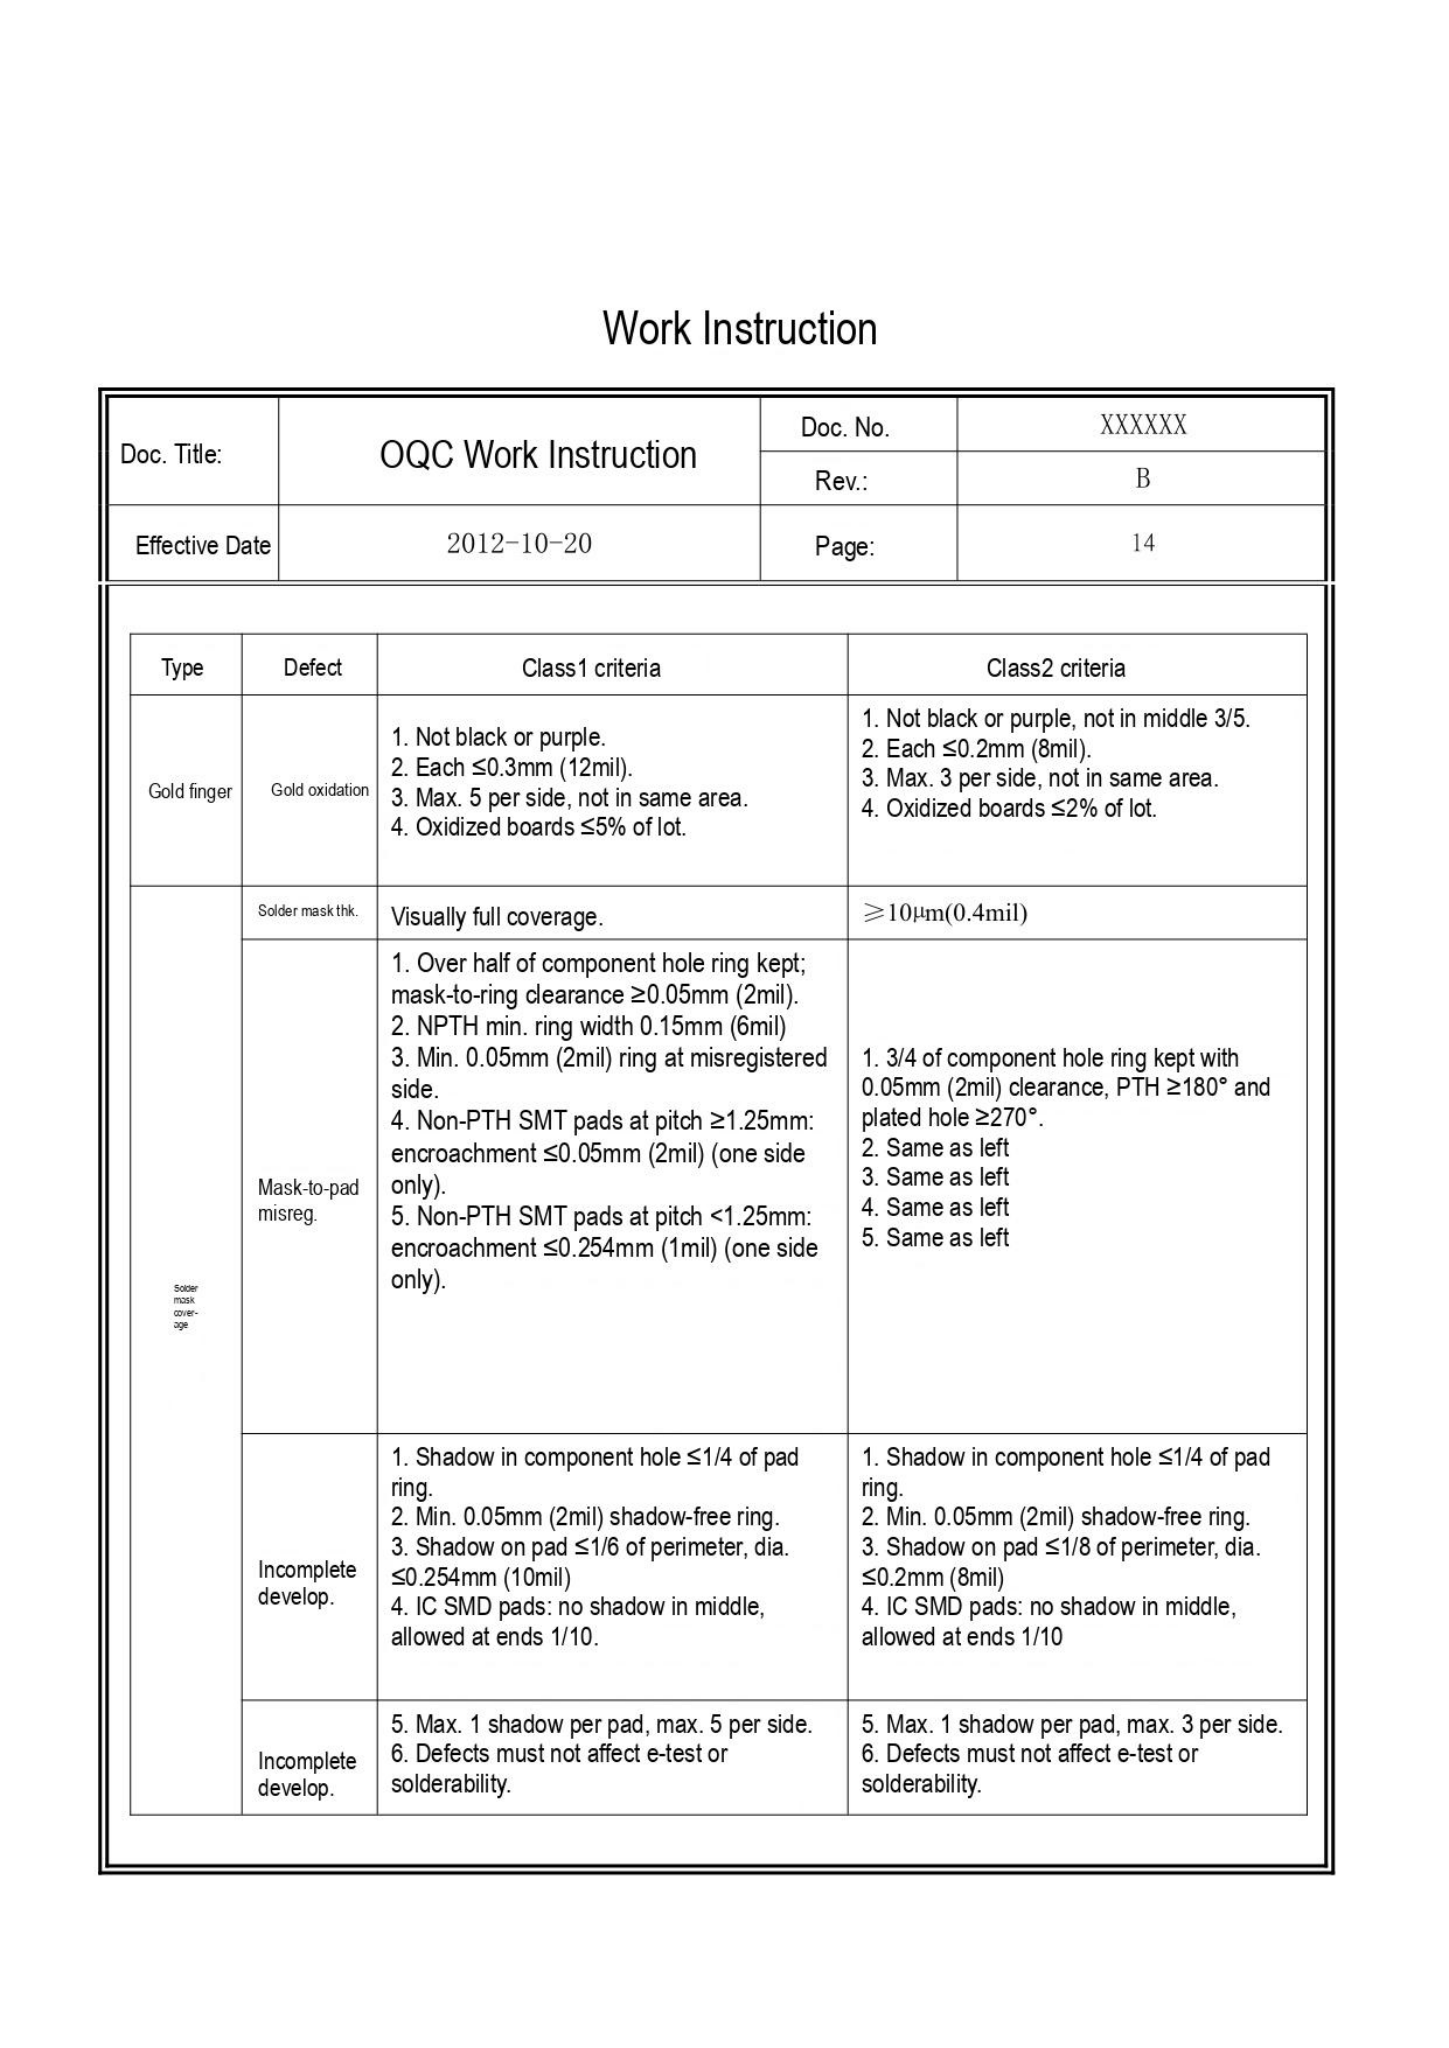Work Instruction

| Doc. Title: | OQC Work Instruction | Doc. No. | XXXXXX |
|---|---|---|---|
| | | Rev.: | B |
| Effective Date | 2012-10-20 | Page: | 14 |

| Type | Defect | Class1 criteria | Class2 criteria |
|---|---|---|---|
| Gold finger | Gold oxidation | 1. Not black or purple.<br>2. Each ≤0.3mm (12mil).<br>3. Max. 5 per side, not in same area.<br>4. Oxidized boards ≤5% of lot. | 1. Not black or purple, not in middle 3/5.<br>2. Each ≤0.2mm (8mil).<br>3. Max. 3 per side, not in same area.<br>4. Oxidized boards ≤2% of lot. |
| Solder mask cover-age | Solder mask thk. | Visually full coverage. | ≥10μm(0.4mil) |
| | Mask-to-pad misreg. | 1. Over half of component hole ring kept; mask-to-ring clearance ≥0.05mm (2mil).<br>2. NPTH min. ring width 0.15mm (6mil)<br>3. Min. 0.05mm (2mil) ring at misregistered side.<br>4. Non-PTH SMT pads at pitch ≥1.25mm: encroachment ≤0.05mm (2mil) (one side only).<br>5. Non-PTH SMT pads at pitch <1.25mm: encroachment ≤0.254mm (1mil) (one side only). | 1. 3/4 of component hole ring kept with 0.05mm (2mil) clearance, PTH ≥180° and plated hole ≥270°.<br>2. Same as left<br>3. Same as left<br>4. Same as left<br>5. Same as left |
| | Incomplete develop. | 1. Shadow in component hole ≤1/4 of pad ring.<br>2. Min. 0.05mm (2mil) shadow-free ring.<br>3. Shadow on pad ≤1/6 of perimeter, dia. ≤0.254mm (10mil)<br>4. IC SMD pads: no shadow in middle, allowed at ends 1/10. | 1. Shadow in component hole ≤1/4 of pad ring.<br>2. Min. 0.05mm (2mil) shadow-free ring.<br>3. Shadow on pad ≤1/8 of perimeter, dia. ≤0.2mm (8mil)<br>4. IC SMD pads: no shadow in middle, allowed at ends 1/10 |
| | Incomplete develop. | 5. Max. 1 shadow per pad, max. 5 per side.<br>6. Defects must not affect e-test or solderability. | 5. Max. 1 shadow per pad, max. 3 per side.<br>6. Defects must not affect e-test or solderability. |
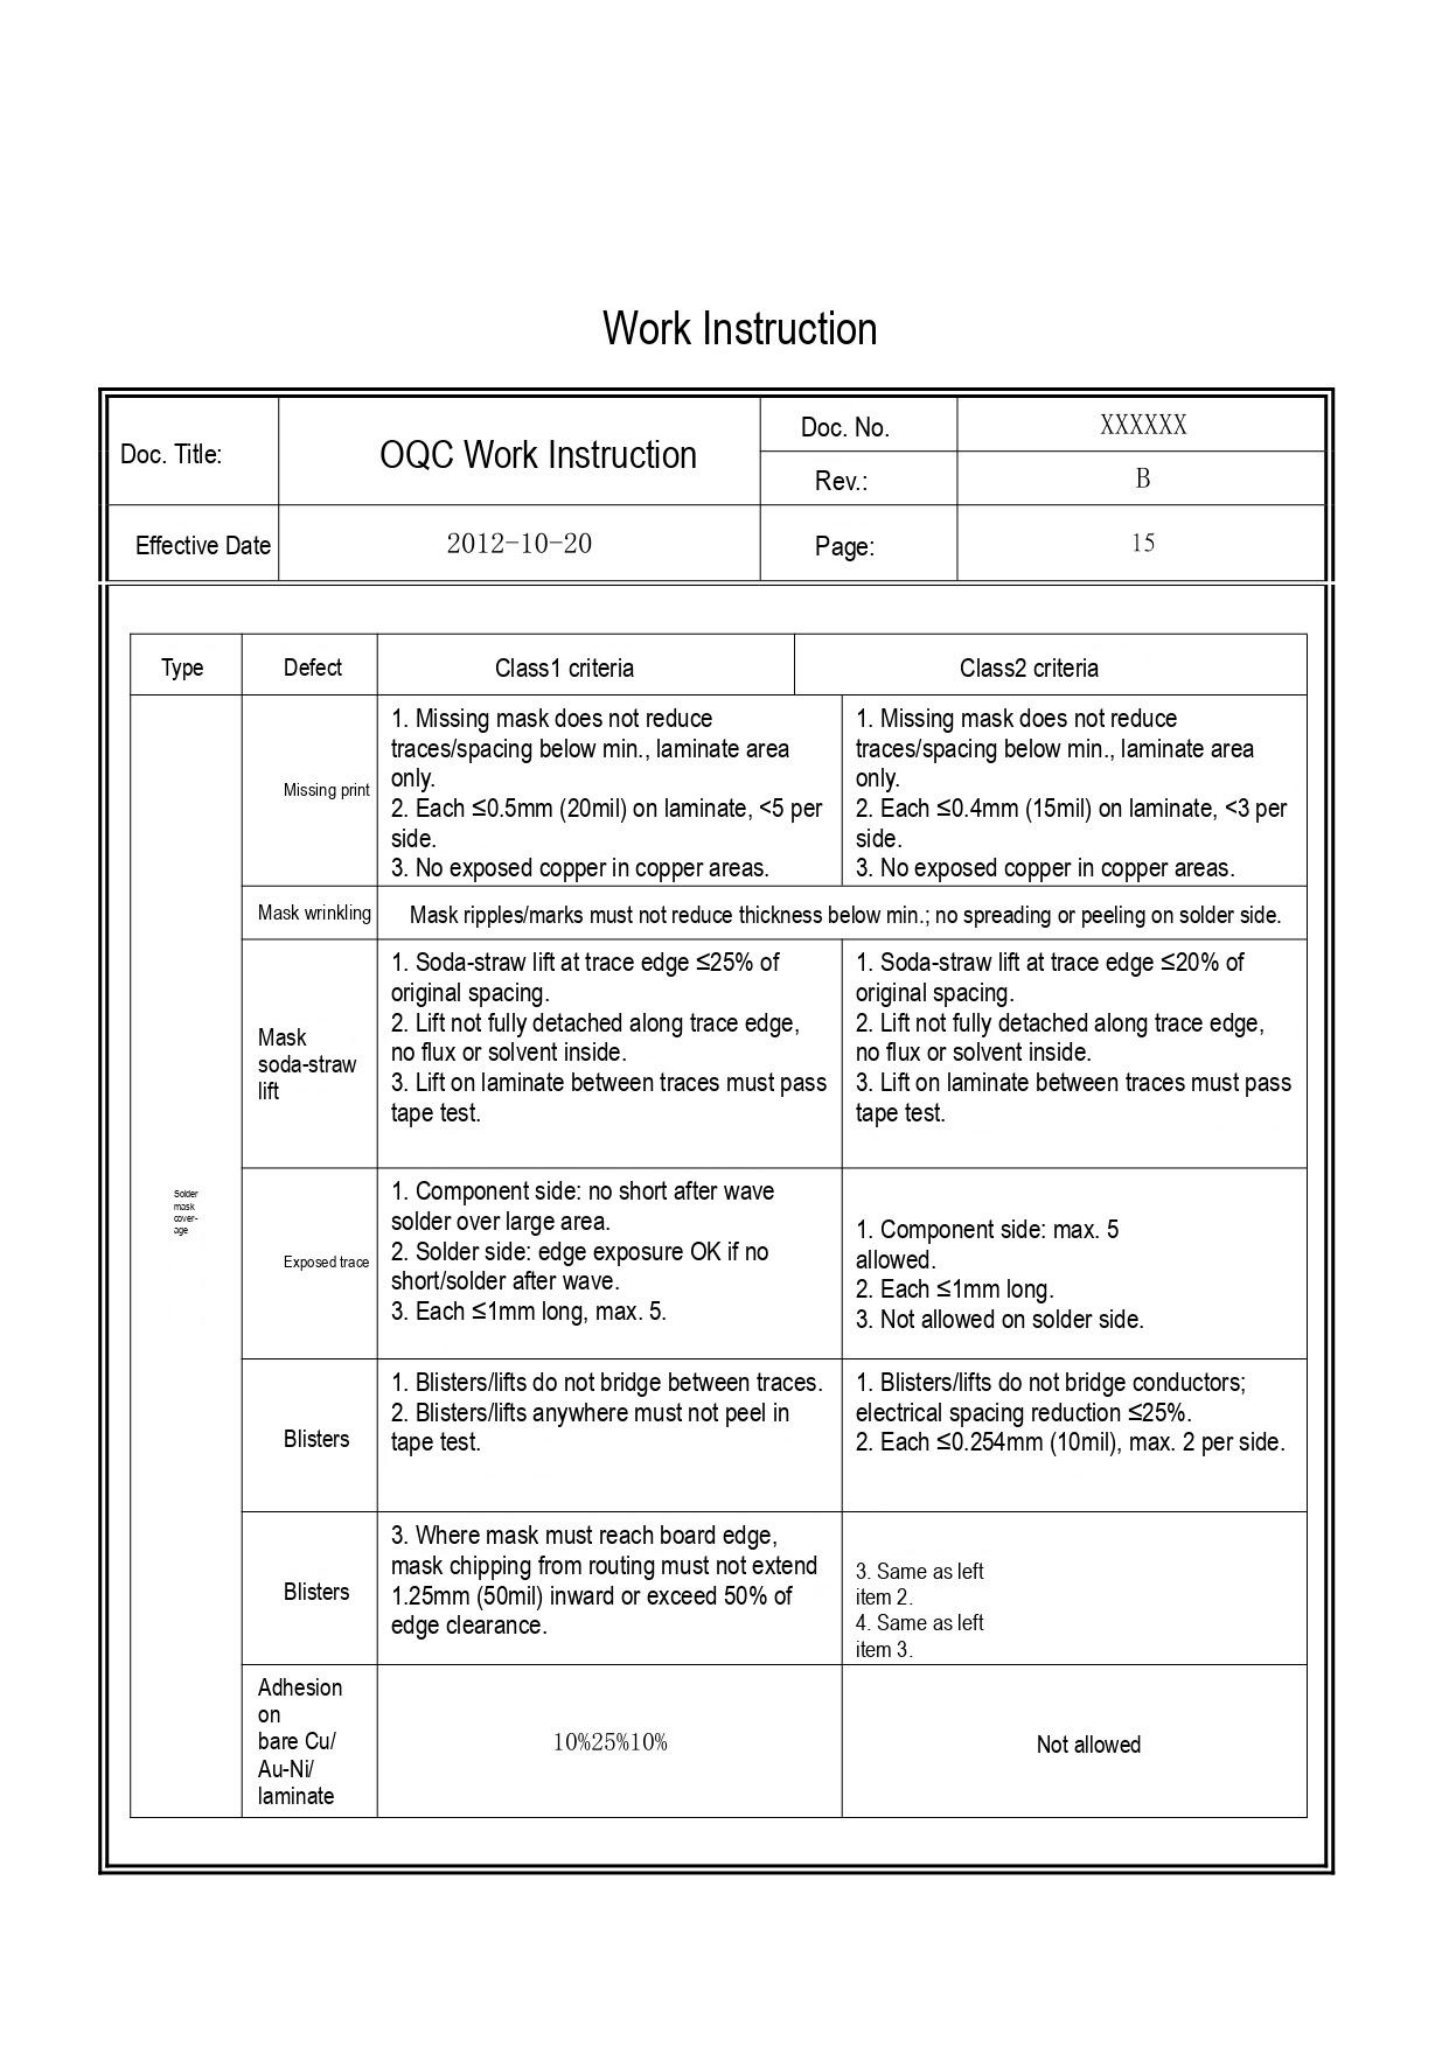Work Instruction

| Doc. Title: | OQC Work Instruction | Doc. No. | XXXXXX |
|---|---|---|---|
| | | Rev.: | B |
| Effective Date | 2012-10-20 | Page: | 15 |

| Type | Defect | Class1 criteria | Class2 criteria |
|---|---|---|---|
| Solder mask cover-age | Missing print | 1. Missing mask does not reduce traces/spacing below min., laminate area only.<br>2. Each ≤0.5mm (20mil) on laminate, <5 per side.<br>3. No exposed copper in copper areas. | 1. Missing mask does not reduce traces/spacing below min., laminate area only.<br>2. Each ≤0.4mm (15mil) on laminate, <3 per side.<br>3. No exposed copper in copper areas. |
| | Mask wrinkling | Mask ripples/marks must not reduce thickness below min.; no spreading or peeling on solder side. | |
| | Mask soda-straw lift | 1. Soda-straw lift at trace edge ≤25% of original spacing.<br>2. Lift not fully detached along trace edge, no flux or solvent inside.<br>3. Lift on laminate between traces must pass tape test. | 1. Soda-straw lift at trace edge ≤20% of original spacing.<br>2. Lift not fully detached along trace edge, no flux or solvent inside.<br>3. Lift on laminate between traces must pass tape test. |
| | Exposed trace | 1. Component side: no short after wave solder over large area.<br>2. Solder side: edge exposure OK if no short/solder after wave.<br>3. Each ≤1mm long, max. 5. | 1. Component side: max. 5 allowed.<br>2. Each ≤1mm long.<br>3. Not allowed on solder side. |
| | Blisters | 1. Blisters/lifts do not bridge between traces.<br>2. Blisters/lifts anywhere must not peel in tape test. | 1. Blisters/lifts do not bridge conductors; electrical spacing reduction ≤25%.<br>2. Each ≤0.254mm (10mil), max. 2 per side. |
| | Blisters | 3. Where mask must reach board edge, mask chipping from routing must not extend 1.25mm (50mil) inward or exceed 50% of edge clearance. | 3. Same as left item 2.<br>4. Same as left item 3. |
| | Adhesion on bare Cu/ Au-Ni/ laminate | 10%25%10% | Not allowed |
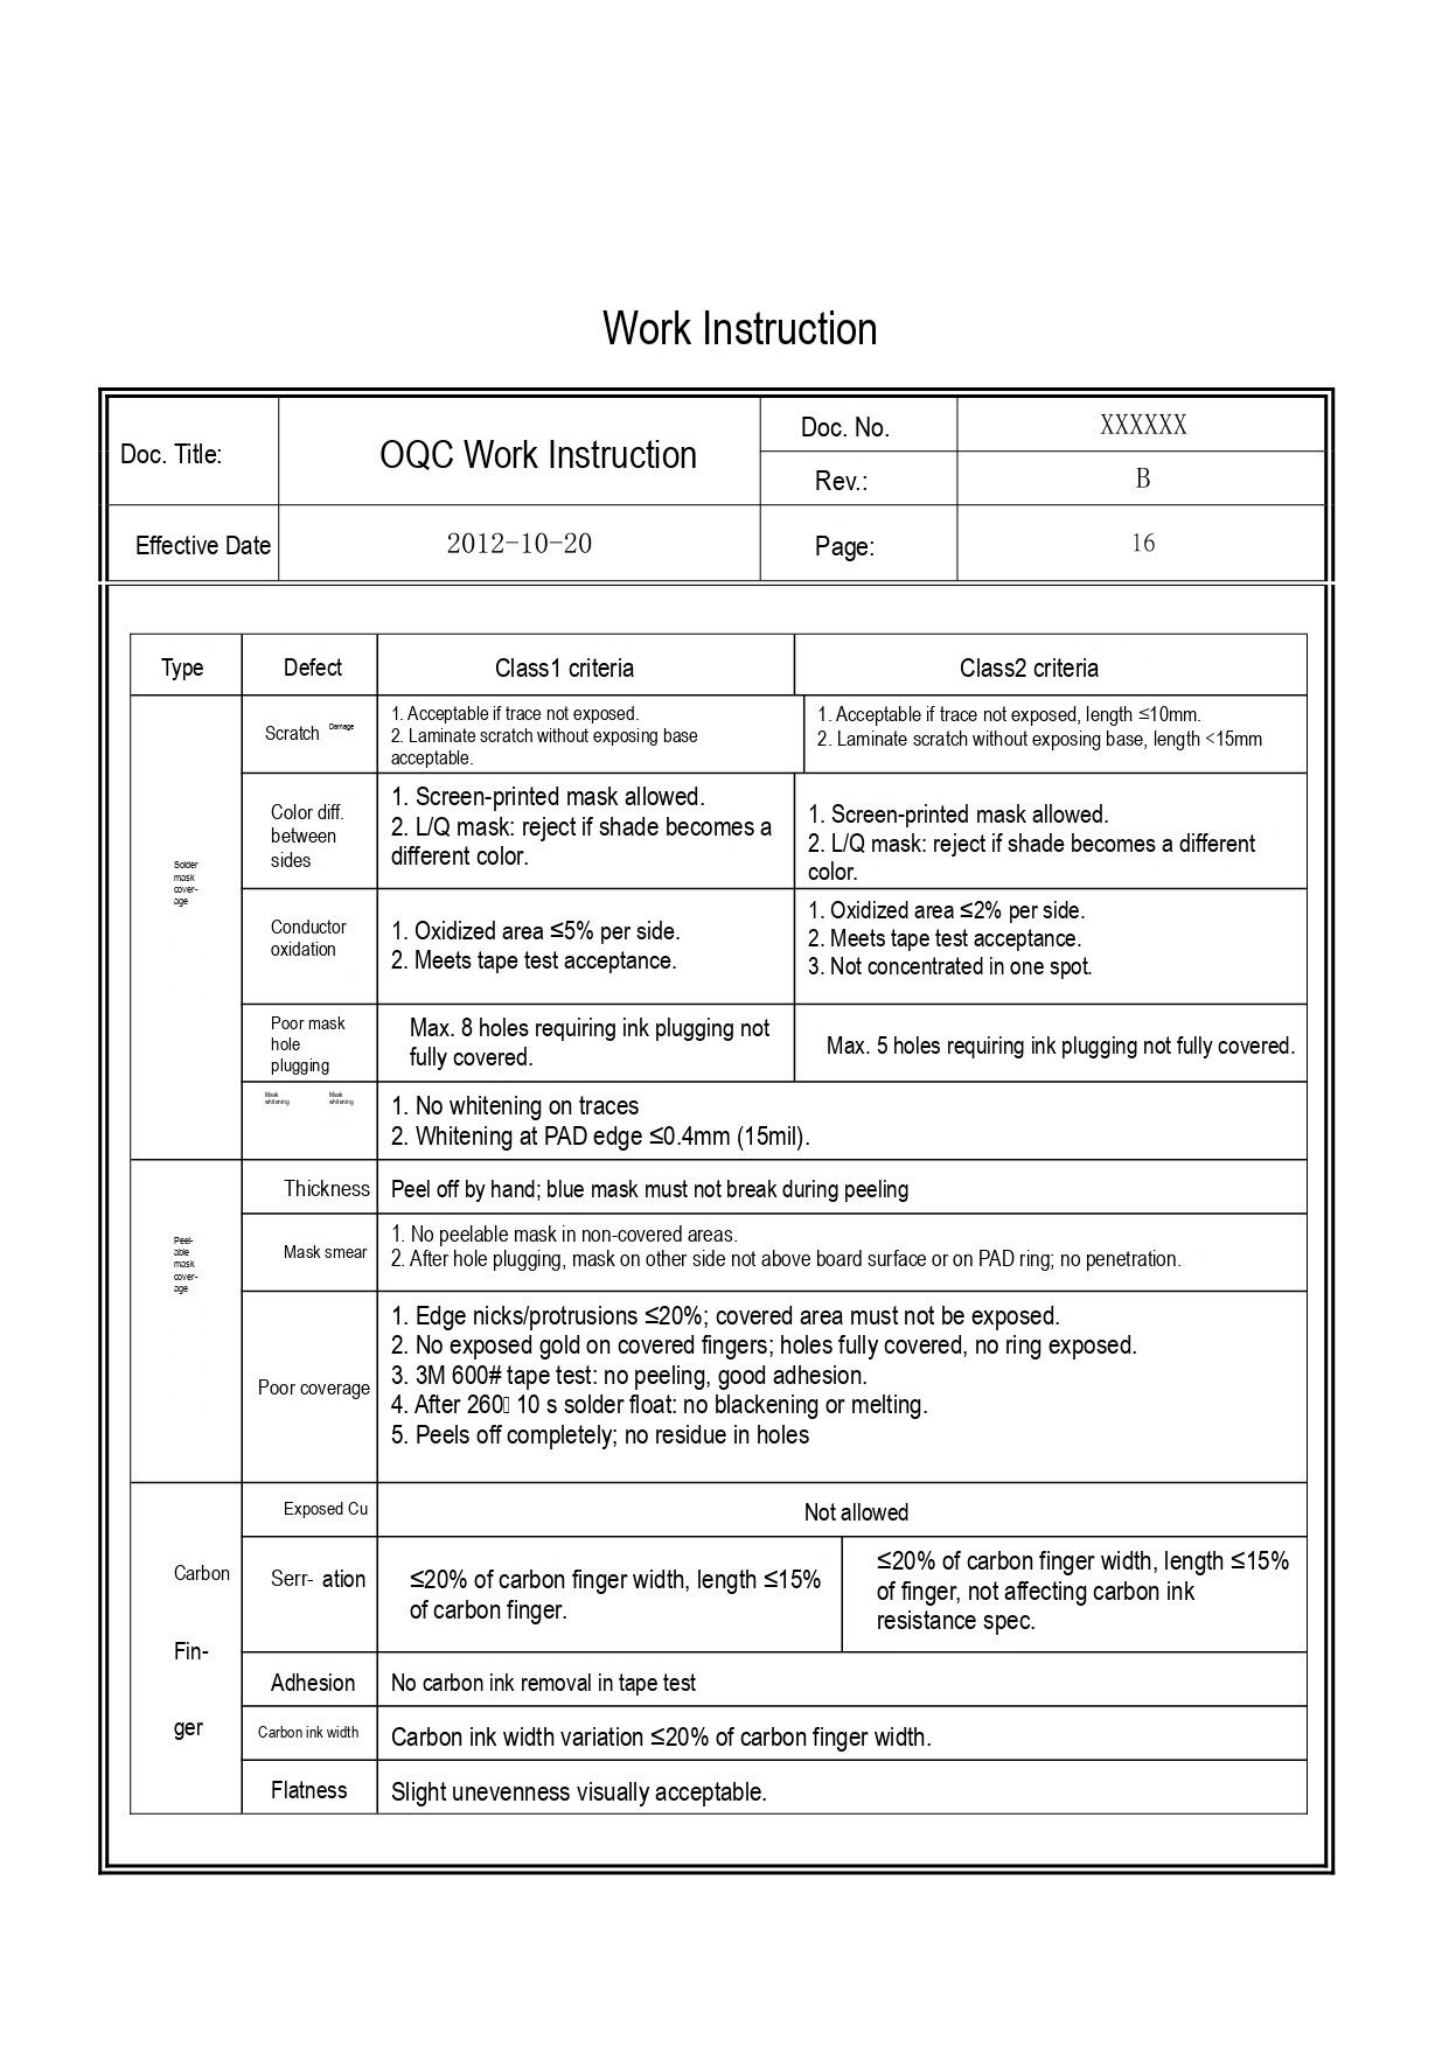Work Instruction

| Doc. Title: | OQC Work Instruction | Doc. No. | XXXXXX |
|---|---|---|---|
| | | Rev.: | B |
| Effective Date | 2012-10-20 | Page: | 16 |

| Type | Defect | Class1 criteria | Class2 criteria |
|---|---|---|---|
| Solder mask cover-age | Scratch Damage | 1. Acceptable if trace not exposed.<br>2. Laminate scratch without exposing base acceptable. | 1. Acceptable if trace not exposed, length ≤10mm.<br>2. Laminate scratch without exposing base, length <15mm |
| | Color diff. between sides | 1. Screen-printed mask allowed.<br>2. L/Q mask: reject if shade becomes a different color. | 1. Screen-printed mask allowed.<br>2. L/Q mask: reject if shade becomes a different color. |
| | Conductor oxidation | 1. Oxidized area ≤5% per side.<br>2. Meets tape test acceptance. | 1. Oxidized area ≤2% per side.<br>2. Meets tape test acceptance.<br>3. Not concentrated in one spot. |
| | Poor mask hole plugging | Max. 8 holes requiring ink plugging not fully covered. | Max. 5 holes requiring ink plugging not fully covered. |
| | Mask whitening Mask whitening | 1. No whitening on traces<br>2. Whitening at PAD edge ≤0.4mm (15mil). | |
| Peel-able mask cover-age | Thickness | Peel off by hand; blue mask must not break during peeling | |
| | Mask smear | 1. No peelable mask in non-covered areas.<br>2. After hole plugging, mask on other side not above board surface or on PAD ring; no penetration. | |
| | Poor coverage | 1. Edge nicks/protrusions ≤20%; covered area must not be exposed.<br>2. No exposed gold on covered fingers; holes fully covered, no ring exposed.<br>3. 3M 600# tape test: no peeling, good adhesion.<br>4. After 260 10 s solder float: no blackening or melting.<br>5. Peels off completely; no residue in holes | |
| Carbon Fin-ger | Exposed Cu | Not allowed | |
| | Serr- ation | ≤20% of carbon finger width, length ≤15% of carbon finger. | ≤20% of carbon finger width, length ≤15% of finger, not affecting carbon ink resistance spec. |
| | Adhesion | No carbon ink removal in tape test | |
| | Carbon ink width | Carbon ink width variation ≤20% of carbon finger width. | |
| | Flatness | Slight unevenness visually acceptable. | |
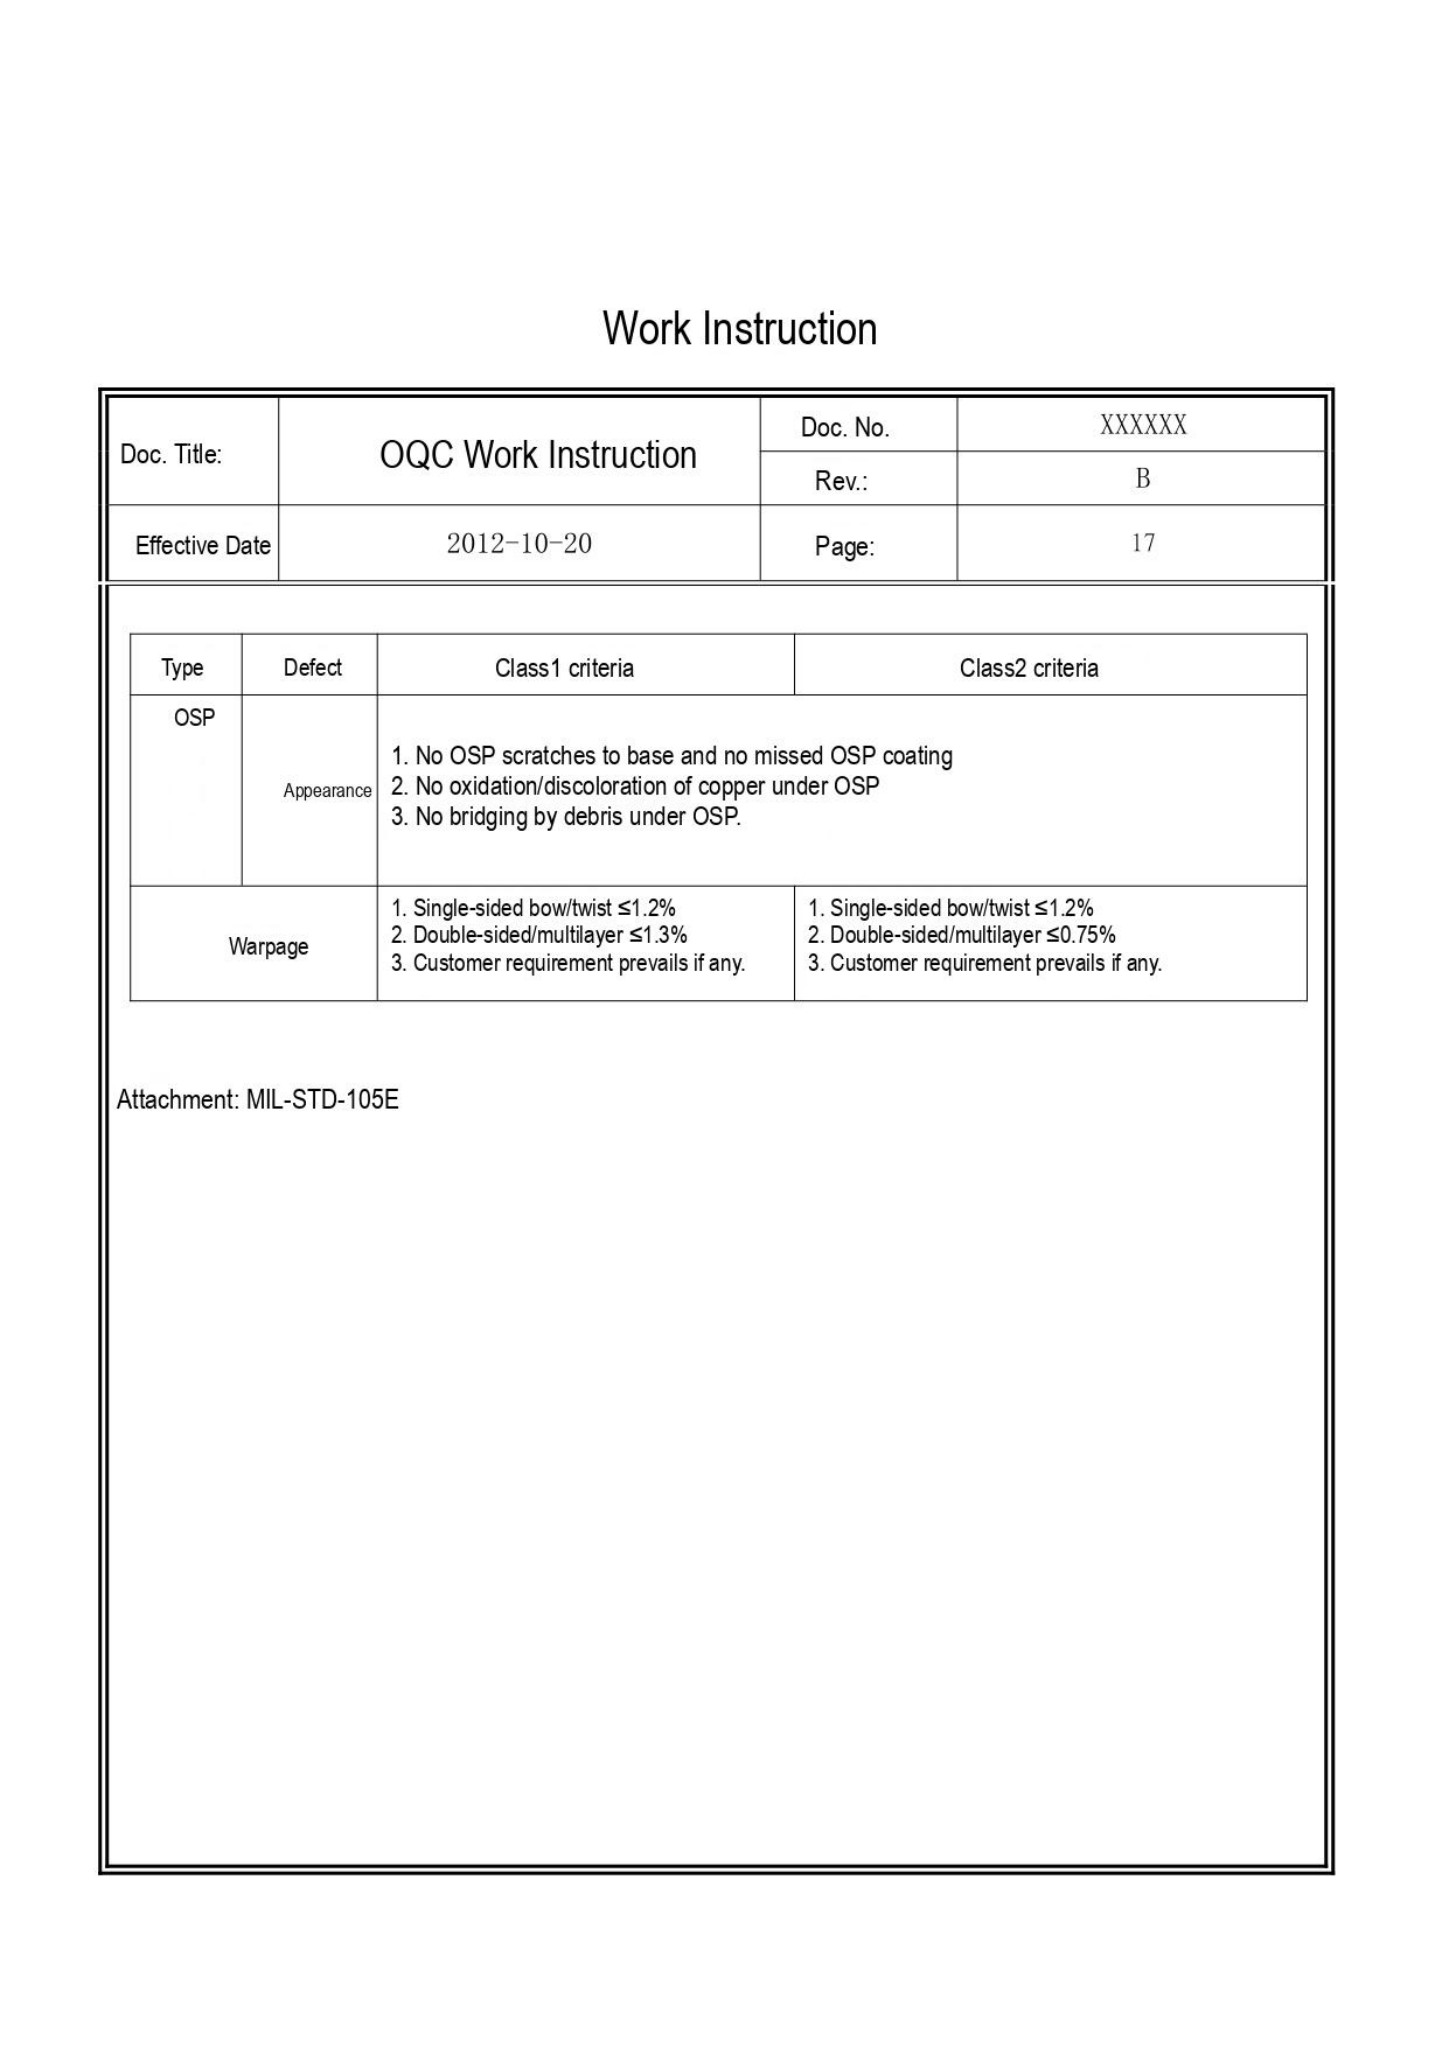Work Instruction

| Doc. Title: | OQC Work Instruction | Doc. No. | XXXXXX |
|---|---|---|---|
| | | Rev.: | B |
| Effective Date | 2012-10-20 | Page: | 17 |

| Type | Defect | Class1 criteria | Class2 criteria |
|---|---|---|---|
| OSP | Appearance | 1. No OSP scratches to base and no missed OSP coating<br>2. No oxidation/discoloration of copper under OSP<br>3. No bridging by debris under OSP. | |
| Warpage | | 1. Single-sided bow/twist ≤1.2%<br>2. Double-sided/multilayer ≤1.3%<br>3. Customer requirement prevails if any. | 1. Single-sided bow/twist ≤1.2%<br>2. Double-sided/multilayer ≤0.75%<br>3. Customer requirement prevails if any. |

Attachment: MIL-STD-105E
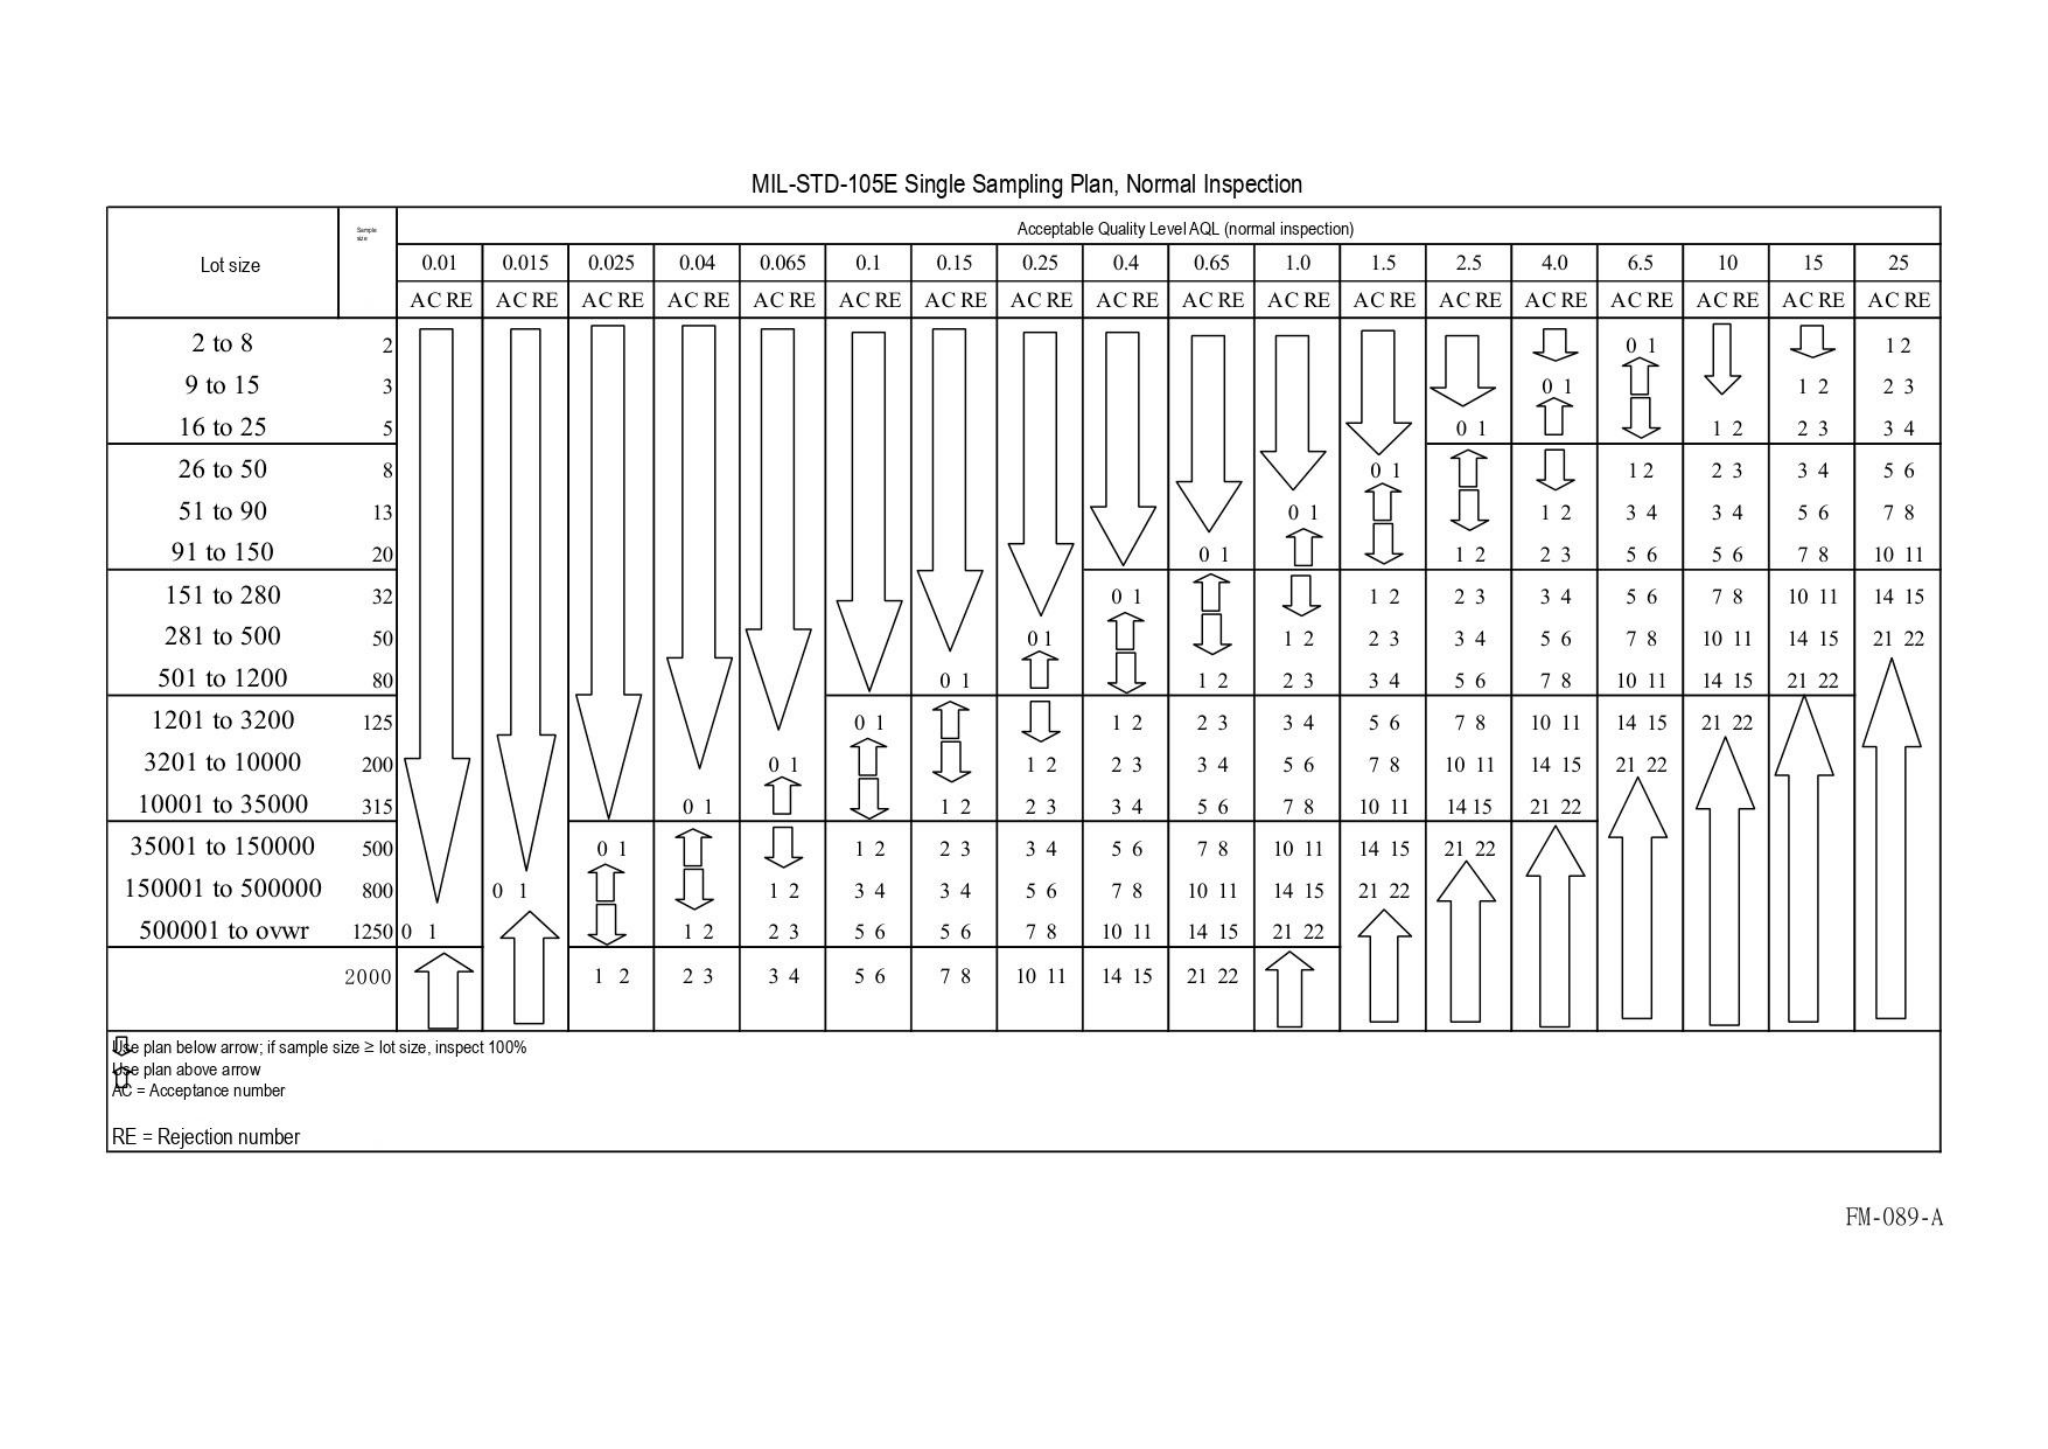MIL-STD-105E Single Sampling Plan, Normal Inspection

| Lot size | Sample size | 0.01 | 0.015 | 0.025 | 0.04 | 0.065 | 0.1 | 0.15 | 0.25 | 0.4 | 0.65 | 1.0 | 1.5 | 2.5 | 4.0 | 6.5 | 10 | 15 | 25 |
|---|---|---|---|---|---|---|---|---|---|---|---|---|---|---|---|---|---|---|---|
| | | Acceptable Quality Level AQL (normal inspection) | | | | | | | | | | | | | | | | | |
| | | AC RE | AC RE | AC RE | AC RE | AC RE | AC RE | AC RE | AC RE | AC RE | AC RE | AC RE | AC RE | AC RE | AC RE | AC RE | AC RE | AC RE | AC RE |
| 2 to 8 | 2 | | | | | | | | | | | | | | | 0 1 | | | 1 2 |
| 9 to 15 | 3 | | | | | | | | | | | | | | 0 1 | | | 1 2 | 2 3 |
| 16 to 25 | 5 | | | | | | | | | | | | | 0 1 | | | 1 2 | 2 3 | 3 4 |
| 26 to 50 | 8 | | | | | | | | | | | | 0 1 | | | 1 2 | 2 3 | 3 4 | 5 6 |
| 51 to 90 | 13 | | | | | | | | | | | 0 1 | | | 1 2 | 3 4 | 3 4 | 5 6 | 7 8 |
| 91 to 150 | 20 | | | | | | | | | | 0 1 | | | 1 2 | 2 3 | 5 6 | 5 6 | 7 8 | 10 11 |
| 151 to 280 | 32 | | | | | | | | | 0 1 | | | 1 2 | 2 3 | 3 4 | 5 6 | 7 8 | 10 11 | 14 15 |
| 281 to 500 | 50 | | | | | | | | 0 1 | | | 1 2 | 2 3 | 3 4 | 5 6 | 7 8 | 10 11 | 14 15 | 21 22 |
| 501 to 1200 | 80 | | | | | | | 0 1 | | | 1 2 | 2 3 | 3 4 | 5 6 | 7 8 | 10 11 | 14 15 | 21 22 | |
| 1201 to 3200 | 125 | | | | | | 0 1 | | | 1 2 | 2 3 | 3 4 | 5 6 | 7 8 | 10 11 | 14 15 | 21 22 | | |
| 3201 to 10000 | 200 | | | | | 0 1 | | | 1 2 | 2 3 | 3 4 | 5 6 | 7 8 | 10 11 | 14 15 | 21 22 | | | |
| 10001 to 35000 | 315 | | | | 0 1 | | | 1 2 | 2 3 | 3 4 | 5 6 | 7 8 | 10 11 | 14 15 | 21 22 | | | | |
| 35001 to 150000 | 500 | | | 0 1 | | | 1 2 | 2 3 | 3 4 | 5 6 | 7 8 | 10 11 | 14 15 | 21 22 | | | | | |
| 150001 to 500000 | 800 | | 0 1 | | | 1 2 | 3 4 | 3 4 | 5 6 | 7 8 | 10 11 | 14 15 | 21 22 | | | | | | |
| 500001 to ovwr | 1250 | 0 1 | | | 1 2 | 2 3 | 5 6 | 5 6 | 7 8 | 10 11 | 14 15 | 21 22 | | | | | | | |
| | 2000 | | | 1 2 | 2 3 | 3 4 | 5 6 | 7 8 | 10 11 | 14 15 | 21 22 | | | | | | | | |

Use plan below arrow; if sample size ≥ lot size, inspect 100%
Use plan above arrow
AC = Acceptance number

RE = Rejection number

FM-089-A